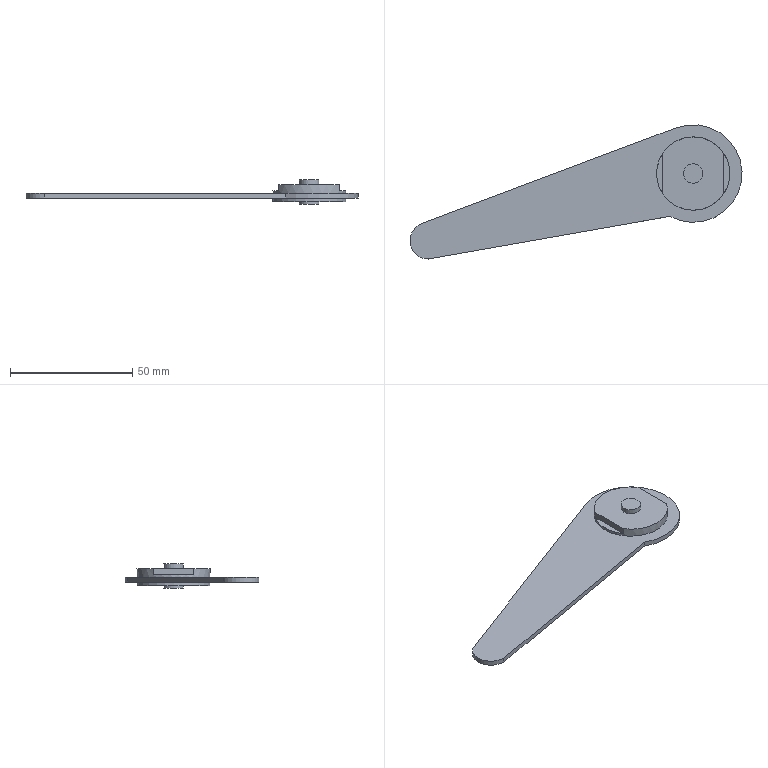Part | NX | 1 solid | 18 faces | box 136 x 55 x 10 mm | volume 10744 mm3 | plane 12 | cylinder 6 | commonest cylinder face diameters 8 x2 30 x2 15 x1 40 x1
STEP:
#1=CARTESIAN_POINT('',(-2.643,7.019,1.));
#2=VERTEX_POINT('',#1);
#3=CARTESIAN_POINT('',(0.,-7.5,1.));
#4=VERTEX_POINT('',#3);
#5=CARTESIAN_POINT('',(0.,0.,1.));
#6=DIRECTION('',(0.,0.,1.));
#7=DIRECTION('',(1.,0.,0.));
#8=AXIS2_PLACEMENT_3D('',#5,#6,#7);
#9=CIRCLE('',#8,7.5);
#10=EDGE_CURVE('',#2,#4,#9,.T.);
#11=ORIENTED_EDGE('',*,*,#10,.T.);
#12=CARTESIAN_POINT('',(98.922,9.943,1.));
#13=VERTEX_POINT('',#12);
#14=CARTESIAN_POINT('',(0.,-7.5,1.));
#15=DIRECTION('',(0.9848,0.1736,0.));
#16=VECTOR('',#15,1000.);
#17=LINE('',#14,#16);
#18=EDGE_CURVE('',#4,#13,#17,.T.);
#19=ORIENTED_EDGE('',*,*,#18,.T.);
#20=CARTESIAN_POINT('',(101.452,46.217,1.));
#21=VERTEX_POINT('',#20);
#22=CARTESIAN_POINT('',(108.5,27.5,1.));
#23=DIRECTION('',(0.,0.,1.));
#24=DIRECTION('',(1.,0.,0.));
#25=AXIS2_PLACEMENT_3D('',#22,#23,#24);
#26=CIRCLE('',#25,20.);
#27=EDGE_CURVE('',#13,#21,#26,.T.);
#28=ORIENTED_EDGE('',*,*,#27,.T.);
#29=CARTESIAN_POINT('',(101.452,46.217,1.));
#30=DIRECTION('',(-0.9358,-0.3524,0.));
#31=VECTOR('',#30,1000.);
#32=LINE('',#29,#31);
#33=EDGE_CURVE('',#21,#2,#32,.T.);
#34=ORIENTED_EDGE('',*,*,#33,.T.);
#35=EDGE_LOOP('',(#11,#19,#28,#34));
#36=FACE_BOUND('',#35,.T.);
#37=CARTESIAN_POINT('',(123.5,27.5,1.));
#38=VERTEX_POINT('',#37);
#39=CARTESIAN_POINT('',(108.5,27.5,1.));
#40=DIRECTION('',(0.,0.,1.));
#41=DIRECTION('',(1.,0.,0.));
#42=AXIS2_PLACEMENT_3D('',#39,#40,#41);
#43=CIRCLE('',#42,15.);
#44=EDGE_CURVE('',#38,#38,#43,.F.);
#45=ORIENTED_EDGE('',*,*,#44,.T.);
#46=EDGE_LOOP('',(#45));
#47=FACE_BOUND('',#46,.T.);
#48=CARTESIAN_POINT('',(0.,0.,1.));
#49=DIRECTION('',(0.,0.,1.));
#50=DIRECTION('',(1.,0.,0.));
#51=AXIS2_PLACEMENT_3D('',#48,#49,#50);
#52=PLANE('',#51);
#53=ADVANCED_FACE('',(#36,#47),#52,.T.);
#54=CARTESIAN_POINT('',(-2.643,7.019,-1.));
#55=VERTEX_POINT('',#54);
#56=CARTESIAN_POINT('',(0.,-7.5,-1.));
#57=VERTEX_POINT('',#56);
#58=CARTESIAN_POINT('',(0.,0.,-1.));
#59=DIRECTION('',(0.,0.,1.));
#60=DIRECTION('',(1.,0.,0.));
#61=AXIS2_PLACEMENT_3D('',#58,#59,#60);
#62=CIRCLE('',#61,7.5);
#63=EDGE_CURVE('',#55,#57,#62,.T.);
#64=ORIENTED_EDGE('',*,*,#63,.F.);
#65=CARTESIAN_POINT('',(101.452,46.217,-1.));
#66=VERTEX_POINT('',#65);
#67=CARTESIAN_POINT('',(101.452,46.217,-1.));
#68=DIRECTION('',(-0.9358,-0.3524,0.));
#69=VECTOR('',#68,1000.);
#70=LINE('',#67,#69);
#71=EDGE_CURVE('',#66,#55,#70,.T.);
#72=ORIENTED_EDGE('',*,*,#71,.F.);
#73=CARTESIAN_POINT('',(98.922,9.943,-1.));
#74=VERTEX_POINT('',#73);
#75=CARTESIAN_POINT('',(108.5,27.5,-1.));
#76=DIRECTION('',(0.,0.,1.));
#77=DIRECTION('',(1.,0.,0.));
#78=AXIS2_PLACEMENT_3D('',#75,#76,#77);
#79=CIRCLE('',#78,20.);
#80=EDGE_CURVE('',#74,#66,#79,.T.);
#81=ORIENTED_EDGE('',*,*,#80,.F.);
#82=CARTESIAN_POINT('',(0.,-7.5,-1.));
#83=DIRECTION('',(0.9848,0.1736,0.));
#84=VECTOR('',#83,1000.);
#85=LINE('',#82,#84);
#86=EDGE_CURVE('',#57,#74,#85,.T.);
#87=ORIENTED_EDGE('',*,*,#86,.F.);
#88=EDGE_LOOP('',(#64,#72,#81,#87));
#89=FACE_BOUND('',#88,.T.);
#90=CARTESIAN_POINT('',(123.5,27.5,-1.));
#91=VERTEX_POINT('',#90);
#92=CARTESIAN_POINT('',(108.5,27.5,-1.));
#93=DIRECTION('',(0.,0.,1.));
#94=DIRECTION('',(1.,0.,0.));
#95=AXIS2_PLACEMENT_3D('',#92,#93,#94);
#96=CIRCLE('',#95,15.);
#97=EDGE_CURVE('',#91,#91,#96,.F.);
#98=ORIENTED_EDGE('',*,*,#97,.F.);
#99=EDGE_LOOP('',(#98));
#100=FACE_BOUND('',#99,.T.);
#101=CARTESIAN_POINT('',(0.,0.,-1.));
#102=DIRECTION('',(0.,0.,1.));
#103=DIRECTION('',(1.,0.,0.));
#104=AXIS2_PLACEMENT_3D('',#101,#102,#103);
#105=PLANE('',#104);
#106=ADVANCED_FACE('',(#89,#100),#105,.F.);
#107=CARTESIAN_POINT('',(-2.643,7.019,1.));
#108=DIRECTION('',(0.,0.,-1.));
#109=VECTOR('',#108,1000.);
#110=LINE('',#107,#109);
#111=EDGE_CURVE('',#2,#55,#110,.T.);
#112=ORIENTED_EDGE('',*,*,#111,.T.);
#113=ORIENTED_EDGE('',*,*,#63,.T.);
#114=CARTESIAN_POINT('',(0.,-7.5,1.));
#115=DIRECTION('',(0.,0.,-1.));
#116=VECTOR('',#115,1000.);
#117=LINE('',#114,#116);
#118=EDGE_CURVE('',#4,#57,#117,.T.);
#119=ORIENTED_EDGE('',*,*,#118,.F.);
#120=ORIENTED_EDGE('',*,*,#10,.F.);
#121=EDGE_LOOP('',(#112,#113,#119,#120));
#122=FACE_BOUND('',#121,.T.);
#123=CARTESIAN_POINT('',(0.,0.,1.));
#124=DIRECTION('',(0.,0.,-1.));
#125=DIRECTION('',(-1.,0.,0.));
#126=AXIS2_PLACEMENT_3D('',#123,#124,#125);
#127=CYLINDRICAL_SURFACE('',#126,7.5);
#128=ADVANCED_FACE('',(#122),#127,.T.);
#129=ORIENTED_EDGE('',*,*,#118,.T.);
#130=ORIENTED_EDGE('',*,*,#86,.T.);
#131=CARTESIAN_POINT('',(98.922,9.943,1.));
#132=DIRECTION('',(0.,0.,-1.));
#133=VECTOR('',#132,1000.);
#134=LINE('',#131,#133);
#135=EDGE_CURVE('',#13,#74,#134,.T.);
#136=ORIENTED_EDGE('',*,*,#135,.F.);
#137=ORIENTED_EDGE('',*,*,#18,.F.);
#138=EDGE_LOOP('',(#129,#130,#136,#137));
#139=FACE_BOUND('',#138,.T.);
#140=CARTESIAN_POINT('',(0.,-7.5,1.));
#141=DIRECTION('',(-0.1736,0.9848,0.));
#142=DIRECTION('',(-0.9848,-0.1736,0.));
#143=AXIS2_PLACEMENT_3D('',#140,#141,#142);
#144=PLANE('',#143);
#145=ADVANCED_FACE('',(#139),#144,.F.);
#146=ORIENTED_EDGE('',*,*,#135,.T.);
#147=ORIENTED_EDGE('',*,*,#80,.T.);
#148=CARTESIAN_POINT('',(101.452,46.217,1.));
#149=DIRECTION('',(0.,0.,-1.));
#150=VECTOR('',#149,1000.);
#151=LINE('',#148,#150);
#152=EDGE_CURVE('',#21,#66,#151,.T.);
#153=ORIENTED_EDGE('',*,*,#152,.F.);
#154=ORIENTED_EDGE('',*,*,#27,.F.);
#155=EDGE_LOOP('',(#146,#147,#153,#154));
#156=FACE_BOUND('',#155,.T.);
#157=CARTESIAN_POINT('',(108.5,27.5,1.));
#158=DIRECTION('',(0.,0.,-1.));
#159=DIRECTION('',(-1.,0.,0.));
#160=AXIS2_PLACEMENT_3D('',#157,#158,#159);
#161=CYLINDRICAL_SURFACE('',#160,20.);
#162=ADVANCED_FACE('',(#156),#161,.T.);
#163=ORIENTED_EDGE('',*,*,#152,.T.);
#164=ORIENTED_EDGE('',*,*,#71,.T.);
#165=ORIENTED_EDGE('',*,*,#111,.F.);
#166=ORIENTED_EDGE('',*,*,#33,.F.);
#167=EDGE_LOOP('',(#163,#164,#165,#166));
#168=FACE_BOUND('',#167,.T.);
#169=CARTESIAN_POINT('',(101.452,46.217,1.));
#170=DIRECTION('',(0.3524,-0.9358,0.));
#171=DIRECTION('',(0.9358,0.3524,0.));
#172=AXIS2_PLACEMENT_3D('',#169,#170,#171);
#173=PLANE('',#172);
#174=ADVANCED_FACE('',(#168),#173,.F.);
#175=CARTESIAN_POINT('',(112.5,27.5,-3.5));
#176=VERTEX_POINT('',#175);
#177=CARTESIAN_POINT('',(108.5,27.5,-3.5));
#178=DIRECTION('',(0.,0.,1.));
#179=DIRECTION('',(1.,0.,0.));
#180=AXIS2_PLACEMENT_3D('',#177,#178,#179);
#181=CIRCLE('',#180,4.);
#182=EDGE_CURVE('',#176,#176,#181,.T.);
#183=ORIENTED_EDGE('',*,*,#182,.F.);
#184=EDGE_LOOP('',(#183));
#185=FACE_BOUND('',#184,.T.);
#186=CARTESIAN_POINT('',(108.5,31.5,-3.5));
#187=DIRECTION('',(0.,0.,1.));
#188=DIRECTION('',(1.,0.,0.));
#189=AXIS2_PLACEMENT_3D('',#186,#187,#188);
#190=PLANE('',#189);
#191=ADVANCED_FACE('',(#185),#190,.F.);
#192=CARTESIAN_POINT('',(112.5,27.5,-2.5));
#193=VERTEX_POINT('',#192);
#194=CARTESIAN_POINT('',(108.5,27.5,-2.5));
#195=DIRECTION('',(0.,0.,1.));
#196=DIRECTION('',(1.,0.,0.));
#197=AXIS2_PLACEMENT_3D('',#194,#195,#196);
#198=CIRCLE('',#197,4.);
#199=EDGE_CURVE('',#193,#193,#198,.T.);
#200=ORIENTED_EDGE('',*,*,#199,.F.);
#201=EDGE_LOOP('',(#200));
#202=FACE_BOUND('',#201,.T.);
#203=ORIENTED_EDGE('',*,*,#182,.T.);
#204=EDGE_LOOP('',(#203));
#205=FACE_BOUND('',#204,.T.);
#206=CARTESIAN_POINT('',(108.5,27.5,-3.5));
#207=DIRECTION('',(0.,0.,1.));
#208=DIRECTION('',(1.,0.,0.));
#209=AXIS2_PLACEMENT_3D('',#206,#207,#208);
#210=CYLINDRICAL_SURFACE('',#209,4.);
#211=ADVANCED_FACE('',(#202,#205),#210,.T.);
#212=CARTESIAN_POINT('',(123.5,27.5,-2.5));
#213=VERTEX_POINT('',#212);
#214=CARTESIAN_POINT('',(108.5,27.5,-2.5));
#215=DIRECTION('',(0.,0.,1.));
#216=DIRECTION('',(1.,0.,0.));
#217=AXIS2_PLACEMENT_3D('',#214,#215,#216);
#218=CIRCLE('',#217,15.);
#219=EDGE_CURVE('',#213,#213,#218,.T.);
#220=ORIENTED_EDGE('',*,*,#219,.F.);
#221=EDGE_LOOP('',(#220));
#222=FACE_BOUND('',#221,.T.);
#223=ORIENTED_EDGE('',*,*,#199,.T.);
#224=EDGE_LOOP('',(#223));
#225=FACE_BOUND('',#224,.T.);
#226=CARTESIAN_POINT('',(108.5,42.5,-2.5));
#227=DIRECTION('',(0.,0.,1.));
#228=DIRECTION('',(1.,0.,0.));
#229=AXIS2_PLACEMENT_3D('',#226,#227,#228);
#230=PLANE('',#229);
#231=ADVANCED_FACE('',(#222,#225),#230,.F.);
#232=ORIENTED_EDGE('',*,*,#219,.T.);
#233=EDGE_LOOP('',(#232));
#234=FACE_BOUND('',#233,.T.);
#235=ORIENTED_EDGE('',*,*,#97,.T.);
#236=EDGE_LOOP('',(#235));
#237=FACE_BOUND('',#236,.T.);
#238=CARTESIAN_POINT('',(108.5,27.5,-3.5));
#239=DIRECTION('',(0.,0.,1.));
#240=DIRECTION('',(1.,0.,0.));
#241=AXIS2_PLACEMENT_3D('',#238,#239,#240);
#242=CYLINDRICAL_SURFACE('',#241,15.);
#243=ADVANCED_FACE('',(#234,#237),#242,.T.);
#244=CARTESIAN_POINT('',(112.5,27.5,6.5));
#245=VERTEX_POINT('',#244);
#246=CARTESIAN_POINT('',(108.5,27.5,6.5));
#247=DIRECTION('',(0.,0.,1.));
#248=DIRECTION('',(1.,0.,0.));
#249=AXIS2_PLACEMENT_3D('',#246,#247,#248);
#250=CIRCLE('',#249,4.);
#251=EDGE_CURVE('',#245,#245,#250,.T.);
#252=ORIENTED_EDGE('',*,*,#251,.T.);
#253=EDGE_LOOP('',(#252));
#254=FACE_BOUND('',#253,.T.);
#255=CARTESIAN_POINT('',(108.5,27.5,6.5));
#256=DIRECTION('',(0.,0.,-1.));
#257=DIRECTION('',(-1.,0.,0.));
#258=AXIS2_PLACEMENT_3D('',#255,#256,#257);
#259=PLANE('',#258);
#260=ADVANCED_FACE('',(#254),#259,.F.);
#261=ORIENTED_EDGE('',*,*,#251,.F.);
#262=EDGE_LOOP('',(#261));
#263=FACE_BOUND('',#262,.T.);
#264=CARTESIAN_POINT('',(112.5,27.5,4.5));
#265=VERTEX_POINT('',#264);
#266=CARTESIAN_POINT('',(108.5,27.5,4.5));
#267=DIRECTION('',(0.,0.,1.));
#268=DIRECTION('',(1.,0.,0.));
#269=AXIS2_PLACEMENT_3D('',#266,#267,#268);
#270=CIRCLE('',#269,4.);
#271=EDGE_CURVE('',#265,#265,#270,.T.);
#272=ORIENTED_EDGE('',*,*,#271,.T.);
#273=EDGE_LOOP('',(#272));
#274=FACE_BOUND('',#273,.T.);
#275=CARTESIAN_POINT('',(108.5,27.5,-3.5));
#276=DIRECTION('',(0.,0.,1.));
#277=DIRECTION('',(1.,0.,0.));
#278=AXIS2_PLACEMENT_3D('',#275,#276,#277);
#279=CYLINDRICAL_SURFACE('',#278,4.);
#280=ADVANCED_FACE('',(#263,#274),#279,.T.);
#281=ORIENTED_EDGE('',*,*,#271,.F.);
#282=EDGE_LOOP('',(#281));
#283=FACE_BOUND('',#282,.T.);
#284=CARTESIAN_POINT('',(121.,35.792,4.5));
#285=VERTEX_POINT('',#284);
#286=CARTESIAN_POINT('',(96.,35.792,4.5));
#287=VERTEX_POINT('',#286);
#288=CARTESIAN_POINT('',(108.5,27.5,4.5));
#289=DIRECTION('',(0.,0.,1.));
#290=DIRECTION('',(1.,0.,0.));
#291=AXIS2_PLACEMENT_3D('',#288,#289,#290);
#292=CIRCLE('',#291,15.);
#293=EDGE_CURVE('',#285,#287,#292,.T.);
#294=ORIENTED_EDGE('',*,*,#293,.T.);
#295=CARTESIAN_POINT('',(96.,19.208,4.5));
#296=VERTEX_POINT('',#295);
#297=CARTESIAN_POINT('',(96.,31.5,4.5));
#298=DIRECTION('',(0.,-1.,0.));
#299=VECTOR('',#298,1000.);
#300=LINE('',#297,#299);
#301=EDGE_CURVE('',#287,#296,#300,.T.);
#302=ORIENTED_EDGE('',*,*,#301,.T.);
#303=CARTESIAN_POINT('',(121.,19.208,4.5));
#304=VERTEX_POINT('',#303);
#305=CARTESIAN_POINT('',(108.5,27.5,4.5));
#306=DIRECTION('',(0.,0.,1.));
#307=DIRECTION('',(1.,0.,0.));
#308=AXIS2_PLACEMENT_3D('',#305,#306,#307);
#309=CIRCLE('',#308,15.);
#310=EDGE_CURVE('',#296,#304,#309,.T.);
#311=ORIENTED_EDGE('',*,*,#310,.T.);
#312=CARTESIAN_POINT('',(121.,31.5,4.5));
#313=DIRECTION('',(0.,1.,0.));
#314=VECTOR('',#313,1000.);
#315=LINE('',#312,#314);
#316=EDGE_CURVE('',#304,#285,#315,.T.);
#317=ORIENTED_EDGE('',*,*,#316,.T.);
#318=EDGE_LOOP('',(#294,#302,#311,#317));
#319=FACE_BOUND('',#318,.T.);
#320=CARTESIAN_POINT('',(108.5,31.5,4.5));
#321=DIRECTION('',(0.,0.,-1.));
#322=DIRECTION('',(-1.,0.,0.));
#323=AXIS2_PLACEMENT_3D('',#320,#321,#322);
#324=PLANE('',#323);
#325=ADVANCED_FACE('',(#283,#319),#324,.F.);
#326=ORIENTED_EDGE('',*,*,#310,.F.);
#327=CARTESIAN_POINT('',(96.,19.208,2.));
#328=VERTEX_POINT('',#327);
#329=CARTESIAN_POINT('',(96.,19.208,-3.5));
#330=DIRECTION('',(0.,0.,1.));
#331=VECTOR('',#330,1000.);
#332=LINE('',#329,#331);
#333=EDGE_CURVE('',#296,#328,#332,.F.);
#334=ORIENTED_EDGE('',*,*,#333,.T.);
#335=CARTESIAN_POINT('',(96.,35.792,2.));
#336=VERTEX_POINT('',#335);
#337=CARTESIAN_POINT('',(108.5,27.5,2.));
#338=DIRECTION('',(0.,0.,1.));
#339=DIRECTION('',(1.,0.,0.));
#340=AXIS2_PLACEMENT_3D('',#337,#338,#339);
#341=CIRCLE('',#340,15.);
#342=EDGE_CURVE('',#336,#328,#341,.T.);
#343=ORIENTED_EDGE('',*,*,#342,.F.);
#344=CARTESIAN_POINT('',(96.,35.792,-3.5));
#345=DIRECTION('',(0.,0.,1.));
#346=VECTOR('',#345,1000.);
#347=LINE('',#344,#346);
#348=EDGE_CURVE('',#336,#287,#347,.T.);
#349=ORIENTED_EDGE('',*,*,#348,.T.);
#350=ORIENTED_EDGE('',*,*,#293,.F.);
#351=CARTESIAN_POINT('',(121.,35.792,2.));
#352=VERTEX_POINT('',#351);
#353=CARTESIAN_POINT('',(121.,35.792,-3.5));
#354=DIRECTION('',(0.,0.,1.));
#355=VECTOR('',#354,1000.);
#356=LINE('',#353,#355);
#357=EDGE_CURVE('',#285,#352,#356,.F.);
#358=ORIENTED_EDGE('',*,*,#357,.T.);
#359=CARTESIAN_POINT('',(121.,19.208,2.));
#360=VERTEX_POINT('',#359);
#361=CARTESIAN_POINT('',(108.5,27.5,2.));
#362=DIRECTION('',(0.,0.,1.));
#363=DIRECTION('',(1.,0.,0.));
#364=AXIS2_PLACEMENT_3D('',#361,#362,#363);
#365=CIRCLE('',#364,15.);
#366=EDGE_CURVE('',#360,#352,#365,.T.);
#367=ORIENTED_EDGE('',*,*,#366,.F.);
#368=CARTESIAN_POINT('',(121.,19.208,-3.5));
#369=DIRECTION('',(0.,0.,1.));
#370=VECTOR('',#369,1000.);
#371=LINE('',#368,#370);
#372=EDGE_CURVE('',#360,#304,#371,.T.);
#373=ORIENTED_EDGE('',*,*,#372,.T.);
#374=EDGE_LOOP('',(#326,#334,#343,#349,#350,#358,#367,#373));
#375=FACE_BOUND('',#374,.T.);
#376=ORIENTED_EDGE('',*,*,#44,.F.);
#377=EDGE_LOOP('',(#376));
#378=FACE_BOUND('',#377,.T.);
#379=CARTESIAN_POINT('',(108.5,27.5,-3.5));
#380=DIRECTION('',(0.,0.,1.));
#381=DIRECTION('',(1.,0.,0.));
#382=AXIS2_PLACEMENT_3D('',#379,#380,#381);
#383=CYLINDRICAL_SURFACE('',#382,15.);
#384=ADVANCED_FACE('',(#375,#378),#383,.T.);
#385=ORIENTED_EDGE('',*,*,#372,.F.);
#386=CARTESIAN_POINT('',(121.,19.208,2.));
#387=DIRECTION('',(0.,1.,0.));
#388=VECTOR('',#387,1000.);
#389=LINE('',#386,#388);
#390=EDGE_CURVE('',#360,#352,#389,.T.);
#391=ORIENTED_EDGE('',*,*,#390,.T.);
#392=ORIENTED_EDGE('',*,*,#357,.F.);
#393=ORIENTED_EDGE('',*,*,#316,.F.);
#394=EDGE_LOOP('',(#385,#391,#392,#393));
#395=FACE_BOUND('',#394,.T.);
#396=CARTESIAN_POINT('',(121.,19.208,5.));
#397=DIRECTION('',(-1.,0.,0.));
#398=DIRECTION('',(0.,0.,1.));
#399=AXIS2_PLACEMENT_3D('',#396,#397,#398);
#400=PLANE('',#399);
#401=ADVANCED_FACE('',(#395),#400,.F.);
#402=ORIENTED_EDGE('',*,*,#366,.T.);
#403=ORIENTED_EDGE('',*,*,#390,.F.);
#404=EDGE_LOOP('',(#402,#403));
#405=FACE_BOUND('',#404,.T.);
#406=CARTESIAN_POINT('',(0.,0.,2.));
#407=DIRECTION('',(0.,0.,1.));
#408=DIRECTION('',(1.,0.,0.));
#409=AXIS2_PLACEMENT_3D('',#406,#407,#408);
#410=PLANE('',#409);
#411=ADVANCED_FACE('',(#405),#410,.T.);
#412=ORIENTED_EDGE('',*,*,#342,.T.);
#413=CARTESIAN_POINT('',(96.,35.792,2.));
#414=DIRECTION('',(0.,-1.,0.));
#415=VECTOR('',#414,1000.);
#416=LINE('',#413,#415);
#417=EDGE_CURVE('',#336,#328,#416,.T.);
#418=ORIENTED_EDGE('',*,*,#417,.F.);
#419=EDGE_LOOP('',(#412,#418));
#420=FACE_BOUND('',#419,.T.);
#421=CARTESIAN_POINT('',(0.,0.,2.));
#422=DIRECTION('',(0.,0.,1.));
#423=DIRECTION('',(1.,0.,0.));
#424=AXIS2_PLACEMENT_3D('',#421,#422,#423);
#425=PLANE('',#424);
#426=ADVANCED_FACE('',(#420),#425,.T.);
#427=ORIENTED_EDGE('',*,*,#348,.F.);
#428=ORIENTED_EDGE('',*,*,#417,.T.);
#429=ORIENTED_EDGE('',*,*,#333,.F.);
#430=ORIENTED_EDGE('',*,*,#301,.F.);
#431=EDGE_LOOP('',(#427,#428,#429,#430));
#432=FACE_BOUND('',#431,.T.);
#433=CARTESIAN_POINT('',(96.,35.792,5.));
#434=DIRECTION('',(1.,0.,0.));
#435=DIRECTION('',(0.,0.,-1.));
#436=AXIS2_PLACEMENT_3D('',#433,#434,#435);
#437=PLANE('',#436);
#438=ADVANCED_FACE('',(#432),#437,.F.);
#439=CLOSED_SHELL('',(#53,#106,#128,#145,#162,#174,#191,#211,#231,#243,#260,#280,#325,#384,#401,#411,#426,#438));
#440=MANIFOLD_SOLID_BREP('',#439);
#441=(LENGTH_UNIT()NAMED_UNIT(*)SI_UNIT(.MILLI.,.METRE.));
#442=UNCERTAINTY_MEASURE_WITH_UNIT(LENGTH_MEASURE(0.00001),#441,'','');
#443=(NAMED_UNIT(*)PLANE_ANGLE_UNIT()SI_UNIT($,.RADIAN.));
#444=(NAMED_UNIT(*)SI_UNIT($,.STERADIAN.)SOLID_ANGLE_UNIT());
#445=(GEOMETRIC_REPRESENTATION_CONTEXT(3)GLOBAL_UNCERTAINTY_ASSIGNED_CONTEXT((#442))GLOBAL_UNIT_ASSIGNED_CONTEXT((#441,#443,#444))REPRESENTATION_CONTEXT('',''));
#446=ADVANCED_BREP_SHAPE_REPRESENTATION('',(#440),#445);